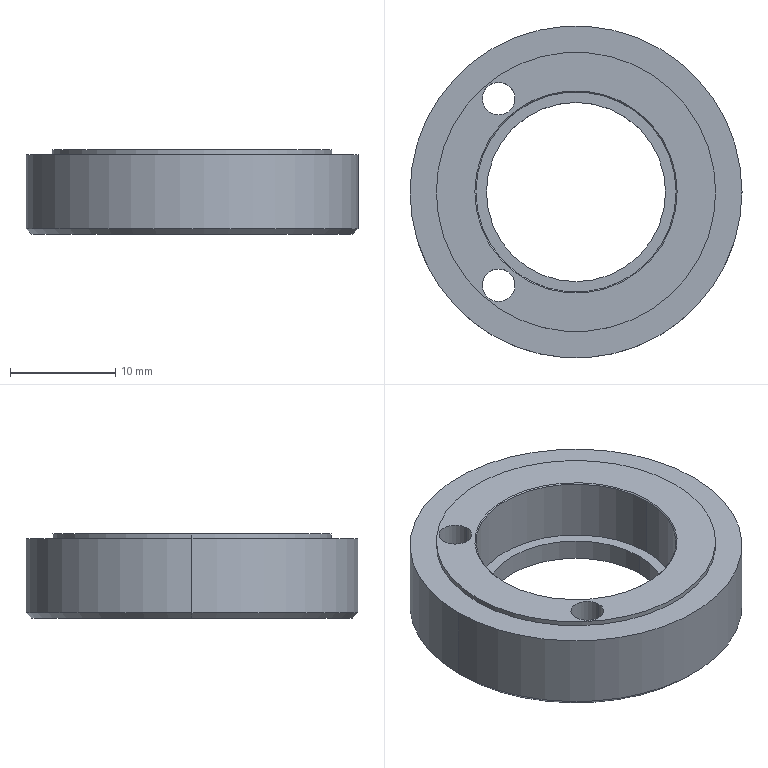Part | SolidWorks | features Chamfer 2, ICE 2, Extrusion 1, HoleWzd 1, MirrorPattern 1 | 1 solid | 20 faces | box 31.5 x 31.5 x 8 mm | volume 3844 mm3 | cylinder 12 | cone 4 | plane 4 | commonest cylinder face diameters 3.1 x4 17 x2 19 x2 26.5 x2 31.5 x2
STEP:
#1=CARTESIAN_POINT('',(-9.5,0.,3.9));
#2=VERTEX_POINT('',#1);
#3=CARTESIAN_POINT('',(9.5,0.,3.9));
#4=VERTEX_POINT('',#3);
#5=CARTESIAN_POINT('',(0.,0.,3.9));
#6=DIRECTION('',(0.,0.,1.));
#7=DIRECTION('',(1.,0.,0.));
#8=AXIS2_PLACEMENT_3D('',#5,#6,#7);
#9=CIRCLE('',#8,9.5);
#10=EDGE_CURVE('',#2,#4,#9,.T.);
#11=ORIENTED_EDGE('',*,*,#10,.F.);
#12=CARTESIAN_POINT('',(-9.6,0.,4.));
#13=VERTEX_POINT('',#12);
#14=CARTESIAN_POINT('',(-9.5,0.,3.9));
#15=DIRECTION('',(-0.7071,0.,0.7071));
#16=VECTOR('',#15,1000.);
#17=LINE('',#14,#16);
#18=EDGE_CURVE('',#2,#13,#17,.T.);
#19=ORIENTED_EDGE('',*,*,#18,.T.);
#20=CARTESIAN_POINT('',(9.6,0.,4.));
#21=VERTEX_POINT('',#20);
#22=CARTESIAN_POINT('',(0.,0.,4.));
#23=DIRECTION('',(0.,0.,-1.));
#24=DIRECTION('',(1.,0.,0.));
#25=AXIS2_PLACEMENT_3D('',#22,#23,#24);
#26=CIRCLE('',#25,9.6);
#27=EDGE_CURVE('',#21,#13,#26,.T.);
#28=ORIENTED_EDGE('',*,*,#27,.F.);
#29=CARTESIAN_POINT('',(9.5,0.,3.9));
#30=DIRECTION('',(0.7071,0.,0.7071));
#31=VECTOR('',#30,1000.);
#32=LINE('',#29,#31);
#33=EDGE_CURVE('',#4,#21,#32,.T.);
#34=ORIENTED_EDGE('',*,*,#33,.F.);
#35=EDGE_LOOP('',(#11,#19,#28,#34));
#36=FACE_OUTER_BOUND('',#35,.T.);
#37=CARTESIAN_POINT('',(0.,0.,3.9));
#38=DIRECTION('',(0.,0.,1.));
#39=DIRECTION('',(1.,0.,0.));
#40=AXIS2_PLACEMENT_3D('',#37,#38,#39);
#41=CONICAL_SURFACE('',#40,9.5,0.7854);
#42=ADVANCED_FACE('',(#36),#41,.F.);
#43=CARTESIAN_POINT('',(-15.25,0.,-4.));
#44=VERTEX_POINT('',#43);
#45=CARTESIAN_POINT('',(15.25,0.,-4.));
#46=VERTEX_POINT('',#45);
#47=CARTESIAN_POINT('',(0.,0.,-4.));
#48=DIRECTION('',(0.,0.,-1.));
#49=DIRECTION('',(1.,0.,0.));
#50=AXIS2_PLACEMENT_3D('',#47,#48,#49);
#51=CIRCLE('',#50,15.25);
#52=EDGE_CURVE('',#44,#46,#51,.T.);
#53=ORIENTED_EDGE('',*,*,#52,.F.);
#54=CARTESIAN_POINT('',(-15.75,0.,-3.5));
#55=VERTEX_POINT('',#54);
#56=CARTESIAN_POINT('',(-15.75,0.,-3.5));
#57=DIRECTION('',(-0.7071,0.,0.7071));
#58=VECTOR('',#57,1000.);
#59=LINE('',#56,#58);
#60=EDGE_CURVE('',#44,#55,#59,.T.);
#61=ORIENTED_EDGE('',*,*,#60,.T.);
#62=CARTESIAN_POINT('',(15.75,0.,-3.5));
#63=VERTEX_POINT('',#62);
#64=CARTESIAN_POINT('',(0.,0.,-3.5));
#65=DIRECTION('',(0.,0.,1.));
#66=DIRECTION('',(1.,0.,0.));
#67=AXIS2_PLACEMENT_3D('',#64,#65,#66);
#68=CIRCLE('',#67,15.75);
#69=EDGE_CURVE('',#63,#55,#68,.T.);
#70=ORIENTED_EDGE('',*,*,#69,.F.);
#71=CARTESIAN_POINT('',(15.75,0.,-3.5));
#72=DIRECTION('',(0.7071,0.,0.7071));
#73=VECTOR('',#72,1000.);
#74=LINE('',#71,#73);
#75=EDGE_CURVE('',#46,#63,#74,.T.);
#76=ORIENTED_EDGE('',*,*,#75,.F.);
#77=EDGE_LOOP('',(#53,#61,#70,#76));
#78=FACE_OUTER_BOUND('',#77,.T.);
#79=CARTESIAN_POINT('',(0.,0.,-3.5));
#80=DIRECTION('',(0.,0.,1.));
#81=DIRECTION('',(1.,0.,0.));
#82=AXIS2_PLACEMENT_3D('',#79,#80,#81);
#83=CONICAL_SURFACE('',#82,15.75,0.7854);
#84=ADVANCED_FACE('',(#78),#83,.T.);
#85=CARTESIAN_POINT('',(13.25,0.,3.55));
#86=VERTEX_POINT('',#85);
#87=CARTESIAN_POINT('',(-13.25,0.,3.55));
#88=VERTEX_POINT('',#87);
#89=CARTESIAN_POINT('',(0.,0.,3.55));
#90=DIRECTION('',(0.,0.,1.));
#91=DIRECTION('',(1.,0.,0.));
#92=AXIS2_PLACEMENT_3D('',#89,#90,#91);
#93=CIRCLE('',#92,13.25);
#94=EDGE_CURVE('',#86,#88,#93,.T.);
#95=ORIENTED_EDGE('',*,*,#94,.T.);
#96=CARTESIAN_POINT('',(-13.25,0.,4.));
#97=VERTEX_POINT('',#96);
#98=CARTESIAN_POINT('',(-13.25,0.,3.55));
#99=DIRECTION('',(0.,0.,1.));
#100=VECTOR('',#99,1000.);
#101=LINE('',#98,#100);
#102=EDGE_CURVE('',#88,#97,#101,.T.);
#103=ORIENTED_EDGE('',*,*,#102,.T.);
#104=CARTESIAN_POINT('',(13.25,0.,4.));
#105=VERTEX_POINT('',#104);
#106=CARTESIAN_POINT('',(0.,0.,4.));
#107=DIRECTION('',(0.,0.,1.));
#108=DIRECTION('',(1.,0.,0.));
#109=AXIS2_PLACEMENT_3D('',#106,#107,#108);
#110=CIRCLE('',#109,13.25);
#111=EDGE_CURVE('',#105,#97,#110,.T.);
#112=ORIENTED_EDGE('',*,*,#111,.F.);
#113=CARTESIAN_POINT('',(13.25,0.,3.55));
#114=DIRECTION('',(0.,0.,1.));
#115=VECTOR('',#114,1000.);
#116=LINE('',#113,#115);
#117=EDGE_CURVE('',#86,#105,#116,.T.);
#118=ORIENTED_EDGE('',*,*,#117,.F.);
#119=EDGE_LOOP('',(#95,#103,#112,#118));
#120=FACE_OUTER_BOUND('',#119,.T.);
#121=CARTESIAN_POINT('',(0.,0.,3.55));
#122=DIRECTION('',(0.,0.,1.));
#123=DIRECTION('',(1.,0.,0.));
#124=AXIS2_PLACEMENT_3D('',#121,#122,#123);
#125=CYLINDRICAL_SURFACE('',#124,13.25);
#126=ADVANCED_FACE('',(#120),#125,.T.);
#127=CARTESIAN_POINT('',(-5.792,-8.852,4.));
#128=VERTEX_POINT('',#127);
#129=CARTESIAN_POINT('',(-8.892,-8.852,4.));
#130=VERTEX_POINT('',#129);
#131=CARTESIAN_POINT('',(-7.342,-8.852,4.));
#132=DIRECTION('',(0.,0.,-1.));
#133=DIRECTION('',(-1.,0.,0.));
#134=AXIS2_PLACEMENT_3D('',#131,#132,#133);
#135=CIRCLE('',#134,1.55);
#136=EDGE_CURVE('',#128,#130,#135,.T.);
#137=ORIENTED_EDGE('',*,*,#136,.F.);
#138=CARTESIAN_POINT('',(-5.792,-8.852,-4.));
#139=VERTEX_POINT('',#138);
#140=CARTESIAN_POINT('',(-5.792,-8.852,-4.));
#141=DIRECTION('',(0.,0.,-1.));
#142=VECTOR('',#141,1000.);
#143=LINE('',#140,#142);
#144=EDGE_CURVE('',#128,#139,#143,.T.);
#145=ORIENTED_EDGE('',*,*,#144,.T.);
#146=CARTESIAN_POINT('',(-8.892,-8.852,-4.));
#147=VERTEX_POINT('',#146);
#148=CARTESIAN_POINT('',(-7.342,-8.852,-4.));
#149=DIRECTION('',(0.,0.,-1.));
#150=DIRECTION('',(-1.,0.,0.));
#151=AXIS2_PLACEMENT_3D('',#148,#149,#150);
#152=CIRCLE('',#151,1.55);
#153=EDGE_CURVE('',#139,#147,#152,.T.);
#154=ORIENTED_EDGE('',*,*,#153,.T.);
#155=CARTESIAN_POINT('',(-8.892,-8.852,-4.));
#156=DIRECTION('',(0.,0.,-1.));
#157=VECTOR('',#156,1000.);
#158=LINE('',#155,#157);
#159=EDGE_CURVE('',#130,#147,#158,.T.);
#160=ORIENTED_EDGE('',*,*,#159,.F.);
#161=EDGE_LOOP('',(#137,#145,#154,#160));
#162=FACE_OUTER_BOUND('',#161,.T.);
#163=CARTESIAN_POINT('',(-7.342,-8.852,-4.));
#164=DIRECTION('',(0.,0.,-1.));
#165=DIRECTION('',(-1.,0.,0.));
#166=AXIS2_PLACEMENT_3D('',#163,#164,#165);
#167=CYLINDRICAL_SURFACE('',#166,1.55);
#168=ADVANCED_FACE('',(#162),#167,.F.);
#169=CARTESIAN_POINT('',(-5.792,8.852,4.));
#170=VERTEX_POINT('',#169);
#171=CARTESIAN_POINT('',(-8.892,8.852,4.));
#172=VERTEX_POINT('',#171);
#173=CARTESIAN_POINT('',(-7.342,8.852,4.));
#174=DIRECTION('',(0.,0.,-1.));
#175=DIRECTION('',(-1.,0.,0.));
#176=AXIS2_PLACEMENT_3D('',#173,#174,#175);
#177=CIRCLE('',#176,1.55);
#178=EDGE_CURVE('',#170,#172,#177,.T.);
#179=ORIENTED_EDGE('',*,*,#178,.F.);
#180=CARTESIAN_POINT('',(-5.792,8.852,-4.));
#181=VERTEX_POINT('',#180);
#182=CARTESIAN_POINT('',(-5.792,8.852,-4.));
#183=DIRECTION('',(0.,0.,-1.));
#184=VECTOR('',#183,1000.);
#185=LINE('',#182,#184);
#186=EDGE_CURVE('',#170,#181,#185,.T.);
#187=ORIENTED_EDGE('',*,*,#186,.T.);
#188=CARTESIAN_POINT('',(-8.892,8.852,-4.));
#189=VERTEX_POINT('',#188);
#190=CARTESIAN_POINT('',(-7.342,8.852,-4.));
#191=DIRECTION('',(0.,0.,-1.));
#192=DIRECTION('',(-1.,0.,0.));
#193=AXIS2_PLACEMENT_3D('',#190,#191,#192);
#194=CIRCLE('',#193,1.55);
#195=EDGE_CURVE('',#181,#189,#194,.T.);
#196=ORIENTED_EDGE('',*,*,#195,.T.);
#197=CARTESIAN_POINT('',(-8.892,8.852,-4.));
#198=DIRECTION('',(0.,0.,-1.));
#199=VECTOR('',#198,1000.);
#200=LINE('',#197,#199);
#201=EDGE_CURVE('',#172,#189,#200,.T.);
#202=ORIENTED_EDGE('',*,*,#201,.F.);
#203=EDGE_LOOP('',(#179,#187,#196,#202));
#204=FACE_OUTER_BOUND('',#203,.T.);
#205=CARTESIAN_POINT('',(-7.342,8.852,-4.));
#206=DIRECTION('',(0.,0.,-1.));
#207=DIRECTION('',(-1.,0.,0.));
#208=AXIS2_PLACEMENT_3D('',#205,#206,#207);
#209=CYLINDRICAL_SURFACE('',#208,1.55);
#210=ADVANCED_FACE('',(#204),#209,.F.);
#211=CARTESIAN_POINT('',(8.5,0.,-2.));
#212=VERTEX_POINT('',#211);
#213=CARTESIAN_POINT('',(-8.5,0.,-2.));
#214=VERTEX_POINT('',#213);
#215=CARTESIAN_POINT('',(0.,0.,-2.));
#216=DIRECTION('',(0.,0.,-1.));
#217=DIRECTION('',(-1.,0.,0.));
#218=AXIS2_PLACEMENT_3D('',#215,#216,#217);
#219=CIRCLE('',#218,8.5);
#220=EDGE_CURVE('',#212,#214,#219,.T.);
#221=ORIENTED_EDGE('',*,*,#220,.F.);
#222=CARTESIAN_POINT('',(8.5,0.,-4.));
#223=VERTEX_POINT('',#222);
#224=CARTESIAN_POINT('',(8.5,0.,-2.));
#225=DIRECTION('',(0.,0.,-1.));
#226=VECTOR('',#225,1000.);
#227=LINE('',#224,#226);
#228=EDGE_CURVE('',#212,#223,#227,.T.);
#229=ORIENTED_EDGE('',*,*,#228,.T.);
#230=CARTESIAN_POINT('',(-8.5,0.,-4.));
#231=VERTEX_POINT('',#230);
#232=CARTESIAN_POINT('',(0.,0.,-4.));
#233=DIRECTION('',(0.,0.,-1.));
#234=DIRECTION('',(-1.,0.,0.));
#235=AXIS2_PLACEMENT_3D('',#232,#233,#234);
#236=CIRCLE('',#235,8.5);
#237=EDGE_CURVE('',#223,#231,#236,.T.);
#238=ORIENTED_EDGE('',*,*,#237,.T.);
#239=CARTESIAN_POINT('',(-8.5,0.,-2.));
#240=DIRECTION('',(0.,0.,-1.));
#241=VECTOR('',#240,1000.);
#242=LINE('',#239,#241);
#243=EDGE_CURVE('',#214,#231,#242,.T.);
#244=ORIENTED_EDGE('',*,*,#243,.F.);
#245=EDGE_LOOP('',(#221,#229,#238,#244));
#246=FACE_OUTER_BOUND('',#245,.T.);
#247=CARTESIAN_POINT('',(0.,0.,-2.));
#248=DIRECTION('',(0.,0.,-1.));
#249=DIRECTION('',(-1.,0.,0.));
#250=AXIS2_PLACEMENT_3D('',#247,#248,#249);
#251=CYLINDRICAL_SURFACE('',#250,8.5);
#252=ADVANCED_FACE('',(#246),#251,.F.);
#253=ORIENTED_EDGE('',*,*,#10,.T.);
#254=CARTESIAN_POINT('',(9.5,0.,-2.));
#255=VERTEX_POINT('',#254);
#256=CARTESIAN_POINT('',(9.5,0.,4.));
#257=DIRECTION('',(0.,0.,-1.));
#258=VECTOR('',#257,1000.);
#259=LINE('',#256,#258);
#260=EDGE_CURVE('',#4,#255,#259,.T.);
#261=ORIENTED_EDGE('',*,*,#260,.T.);
#262=CARTESIAN_POINT('',(-9.5,0.,-2.));
#263=VERTEX_POINT('',#262);
#264=CARTESIAN_POINT('',(0.,0.,-2.));
#265=DIRECTION('',(0.,0.,-1.));
#266=DIRECTION('',(-1.,0.,0.));
#267=AXIS2_PLACEMENT_3D('',#264,#265,#266);
#268=CIRCLE('',#267,9.5);
#269=EDGE_CURVE('',#255,#263,#268,.T.);
#270=ORIENTED_EDGE('',*,*,#269,.T.);
#271=CARTESIAN_POINT('',(-9.5,0.,4.));
#272=DIRECTION('',(0.,0.,-1.));
#273=VECTOR('',#272,1000.);
#274=LINE('',#271,#273);
#275=EDGE_CURVE('',#2,#263,#274,.T.);
#276=ORIENTED_EDGE('',*,*,#275,.F.);
#277=EDGE_LOOP('',(#253,#261,#270,#276));
#278=FACE_OUTER_BOUND('',#277,.T.);
#279=CARTESIAN_POINT('',(0.,0.,4.));
#280=DIRECTION('',(0.,0.,-1.));
#281=DIRECTION('',(-1.,0.,0.));
#282=AXIS2_PLACEMENT_3D('',#279,#280,#281);
#283=CYLINDRICAL_SURFACE('',#282,9.5);
#284=ADVANCED_FACE('',(#278),#283,.F.);
#285=CARTESIAN_POINT('',(15.75,0.,3.55));
#286=VERTEX_POINT('',#285);
#287=CARTESIAN_POINT('',(-15.75,0.,3.55));
#288=VERTEX_POINT('',#287);
#289=CARTESIAN_POINT('',(0.,0.,3.55));
#290=DIRECTION('',(0.,0.,1.));
#291=DIRECTION('',(1.,0.,0.));
#292=AXIS2_PLACEMENT_3D('',#289,#290,#291);
#293=CIRCLE('',#292,15.75);
#294=EDGE_CURVE('',#286,#288,#293,.T.);
#295=ORIENTED_EDGE('',*,*,#294,.F.);
#296=CARTESIAN_POINT('',(15.75,0.,4.));
#297=DIRECTION('',(0.,0.,-1.));
#298=VECTOR('',#297,1000.);
#299=LINE('',#296,#298);
#300=EDGE_CURVE('',#286,#63,#299,.T.);
#301=ORIENTED_EDGE('',*,*,#300,.T.);
#302=ORIENTED_EDGE('',*,*,#69,.T.);
#303=CARTESIAN_POINT('',(-15.75,0.,4.));
#304=DIRECTION('',(0.,0.,-1.));
#305=VECTOR('',#304,1000.);
#306=LINE('',#303,#305);
#307=EDGE_CURVE('',#288,#55,#306,.T.);
#308=ORIENTED_EDGE('',*,*,#307,.F.);
#309=EDGE_LOOP('',(#295,#301,#302,#308));
#310=FACE_OUTER_BOUND('',#309,.T.);
#311=CARTESIAN_POINT('',(0.,0.,4.));
#312=DIRECTION('',(0.,0.,-1.));
#313=DIRECTION('',(-1.,0.,0.));
#314=AXIS2_PLACEMENT_3D('',#311,#312,#313);
#315=CYLINDRICAL_SURFACE('',#314,15.75);
#316=ADVANCED_FACE('',(#310),#315,.T.);
#317=ORIENTED_EDGE('',*,*,#27,.T.);
#318=CARTESIAN_POINT('',(0.,0.,4.));
#319=DIRECTION('',(0.,0.,-1.));
#320=DIRECTION('',(1.,0.,0.));
#321=AXIS2_PLACEMENT_3D('',#318,#319,#320);
#322=CIRCLE('',#321,9.6);
#323=EDGE_CURVE('',#13,#21,#322,.T.);
#324=ORIENTED_EDGE('',*,*,#323,.T.);
#325=EDGE_LOOP('',(#317,#324));
#326=FACE_BOUND('',#325,.T.);
#327=CARTESIAN_POINT('',(-7.342,8.852,4.));
#328=DIRECTION('',(0.,0.,-1.));
#329=DIRECTION('',(-1.,0.,0.));
#330=AXIS2_PLACEMENT_3D('',#327,#328,#329);
#331=CIRCLE('',#330,1.55);
#332=EDGE_CURVE('',#172,#170,#331,.T.);
#333=ORIENTED_EDGE('',*,*,#332,.T.);
#334=ORIENTED_EDGE('',*,*,#178,.T.);
#335=EDGE_LOOP('',(#333,#334));
#336=FACE_BOUND('',#335,.T.);
#337=CARTESIAN_POINT('',(-7.342,-8.852,4.));
#338=DIRECTION('',(0.,0.,-1.));
#339=DIRECTION('',(-1.,0.,0.));
#340=AXIS2_PLACEMENT_3D('',#337,#338,#339);
#341=CIRCLE('',#340,1.55);
#342=EDGE_CURVE('',#130,#128,#341,.T.);
#343=ORIENTED_EDGE('',*,*,#342,.T.);
#344=ORIENTED_EDGE('',*,*,#136,.T.);
#345=EDGE_LOOP('',(#343,#344));
#346=FACE_BOUND('',#345,.T.);
#347=ORIENTED_EDGE('',*,*,#111,.T.);
#348=CARTESIAN_POINT('',(0.,0.,4.));
#349=DIRECTION('',(0.,0.,1.));
#350=DIRECTION('',(1.,0.,0.));
#351=AXIS2_PLACEMENT_3D('',#348,#349,#350);
#352=CIRCLE('',#351,13.25);
#353=EDGE_CURVE('',#97,#105,#352,.T.);
#354=ORIENTED_EDGE('',*,*,#353,.T.);
#355=EDGE_LOOP('',(#347,#354));
#356=FACE_OUTER_BOUND('',#355,.T.);
#357=CARTESIAN_POINT('',(0.,0.,4.));
#358=DIRECTION('',(0.,0.,1.));
#359=DIRECTION('',(1.,0.,0.));
#360=AXIS2_PLACEMENT_3D('',#357,#358,#359);
#361=PLANE('',#360);
#362=ADVANCED_FACE('',(#326,#336,#346,#356),#361,.T.);
#363=ORIENTED_EDGE('',*,*,#300,.F.);
#364=CARTESIAN_POINT('',(0.,0.,3.55));
#365=DIRECTION('',(0.,0.,1.));
#366=DIRECTION('',(1.,0.,0.));
#367=AXIS2_PLACEMENT_3D('',#364,#365,#366);
#368=CIRCLE('',#367,15.75);
#369=EDGE_CURVE('',#288,#286,#368,.T.);
#370=ORIENTED_EDGE('',*,*,#369,.F.);
#371=ORIENTED_EDGE('',*,*,#307,.T.);
#372=CARTESIAN_POINT('',(0.,0.,-3.5));
#373=DIRECTION('',(0.,0.,1.));
#374=DIRECTION('',(1.,0.,0.));
#375=AXIS2_PLACEMENT_3D('',#372,#373,#374);
#376=CIRCLE('',#375,15.75);
#377=EDGE_CURVE('',#55,#63,#376,.T.);
#378=ORIENTED_EDGE('',*,*,#377,.T.);
#379=EDGE_LOOP('',(#363,#370,#371,#378));
#380=FACE_OUTER_BOUND('',#379,.T.);
#381=CARTESIAN_POINT('',(0.,0.,4.));
#382=DIRECTION('',(0.,0.,-1.));
#383=DIRECTION('',(-1.,0.,0.));
#384=AXIS2_PLACEMENT_3D('',#381,#382,#383);
#385=CYLINDRICAL_SURFACE('',#384,15.75);
#386=ADVANCED_FACE('',(#380),#385,.T.);
#387=ORIENTED_EDGE('',*,*,#260,.F.);
#388=CARTESIAN_POINT('',(0.,0.,3.9));
#389=DIRECTION('',(0.,0.,1.));
#390=DIRECTION('',(1.,0.,0.));
#391=AXIS2_PLACEMENT_3D('',#388,#389,#390);
#392=CIRCLE('',#391,9.5);
#393=EDGE_CURVE('',#4,#2,#392,.T.);
#394=ORIENTED_EDGE('',*,*,#393,.T.);
#395=ORIENTED_EDGE('',*,*,#275,.T.);
#396=CARTESIAN_POINT('',(0.,0.,-2.));
#397=DIRECTION('',(0.,0.,-1.));
#398=DIRECTION('',(-1.,0.,0.));
#399=AXIS2_PLACEMENT_3D('',#396,#397,#398);
#400=CIRCLE('',#399,9.5);
#401=EDGE_CURVE('',#263,#255,#400,.T.);
#402=ORIENTED_EDGE('',*,*,#401,.T.);
#403=EDGE_LOOP('',(#387,#394,#395,#402));
#404=FACE_OUTER_BOUND('',#403,.T.);
#405=CARTESIAN_POINT('',(0.,0.,4.));
#406=DIRECTION('',(0.,0.,-1.));
#407=DIRECTION('',(-1.,0.,0.));
#408=AXIS2_PLACEMENT_3D('',#405,#406,#407);
#409=CYLINDRICAL_SURFACE('',#408,9.5);
#410=ADVANCED_FACE('',(#404),#409,.F.);
#411=CARTESIAN_POINT('',(0.,0.,-4.));
#412=DIRECTION('',(0.,0.,-1.));
#413=DIRECTION('',(1.,0.,0.));
#414=AXIS2_PLACEMENT_3D('',#411,#412,#413);
#415=CIRCLE('',#414,15.25);
#416=EDGE_CURVE('',#46,#44,#415,.T.);
#417=ORIENTED_EDGE('',*,*,#416,.T.);
#418=ORIENTED_EDGE('',*,*,#52,.T.);
#419=EDGE_LOOP('',(#417,#418));
#420=FACE_OUTER_BOUND('',#419,.T.);
#421=CARTESIAN_POINT('',(-7.342,-8.852,-4.));
#422=DIRECTION('',(0.,0.,-1.));
#423=DIRECTION('',(-1.,0.,0.));
#424=AXIS2_PLACEMENT_3D('',#421,#422,#423);
#425=CIRCLE('',#424,1.55);
#426=EDGE_CURVE('',#147,#139,#425,.T.);
#427=ORIENTED_EDGE('',*,*,#426,.F.);
#428=ORIENTED_EDGE('',*,*,#153,.F.);
#429=EDGE_LOOP('',(#427,#428));
#430=FACE_BOUND('',#429,.T.);
#431=CARTESIAN_POINT('',(-7.342,8.852,-4.));
#432=DIRECTION('',(0.,0.,-1.));
#433=DIRECTION('',(-1.,0.,0.));
#434=AXIS2_PLACEMENT_3D('',#431,#432,#433);
#435=CIRCLE('',#434,1.55);
#436=EDGE_CURVE('',#189,#181,#435,.T.);
#437=ORIENTED_EDGE('',*,*,#436,.F.);
#438=ORIENTED_EDGE('',*,*,#195,.F.);
#439=EDGE_LOOP('',(#437,#438));
#440=FACE_BOUND('',#439,.T.);
#441=CARTESIAN_POINT('',(0.,0.,-4.));
#442=DIRECTION('',(0.,0.,-1.));
#443=DIRECTION('',(-1.,0.,0.));
#444=AXIS2_PLACEMENT_3D('',#441,#442,#443);
#445=CIRCLE('',#444,8.5);
#446=EDGE_CURVE('',#231,#223,#445,.T.);
#447=ORIENTED_EDGE('',*,*,#446,.F.);
#448=ORIENTED_EDGE('',*,*,#237,.F.);
#449=EDGE_LOOP('',(#447,#448));
#450=FACE_BOUND('',#449,.T.);
#451=CARTESIAN_POINT('',(0.,0.,-4.));
#452=DIRECTION('',(0.,0.,1.));
#453=DIRECTION('',(1.,0.,0.));
#454=AXIS2_PLACEMENT_3D('',#451,#452,#453);
#455=PLANE('',#454);
#456=ADVANCED_FACE('',(#420,#430,#440,#450),#455,.F.);
#457=CARTESIAN_POINT('',(0.,0.,-2.));
#458=DIRECTION('',(0.,0.,-1.));
#459=DIRECTION('',(-1.,0.,0.));
#460=AXIS2_PLACEMENT_3D('',#457,#458,#459);
#461=CIRCLE('',#460,8.5);
#462=EDGE_CURVE('',#214,#212,#461,.T.);
#463=ORIENTED_EDGE('',*,*,#462,.T.);
#464=ORIENTED_EDGE('',*,*,#220,.T.);
#465=EDGE_LOOP('',(#463,#464));
#466=FACE_BOUND('',#465,.T.);
#467=ORIENTED_EDGE('',*,*,#401,.F.);
#468=ORIENTED_EDGE('',*,*,#269,.F.);
#469=EDGE_LOOP('',(#467,#468));
#470=FACE_OUTER_BOUND('',#469,.T.);
#471=CARTESIAN_POINT('',(0.,0.,-2.));
#472=DIRECTION('',(0.,0.,-1.));
#473=DIRECTION('',(-1.,0.,0.));
#474=AXIS2_PLACEMENT_3D('',#471,#472,#473);
#475=PLANE('',#474);
#476=ADVANCED_FACE('',(#466,#470),#475,.F.);
#477=ORIENTED_EDGE('',*,*,#228,.F.);
#478=ORIENTED_EDGE('',*,*,#462,.F.);
#479=ORIENTED_EDGE('',*,*,#243,.T.);
#480=ORIENTED_EDGE('',*,*,#446,.T.);
#481=EDGE_LOOP('',(#477,#478,#479,#480));
#482=FACE_OUTER_BOUND('',#481,.T.);
#483=CARTESIAN_POINT('',(0.,0.,-2.));
#484=DIRECTION('',(0.,0.,-1.));
#485=DIRECTION('',(-1.,0.,0.));
#486=AXIS2_PLACEMENT_3D('',#483,#484,#485);
#487=CYLINDRICAL_SURFACE('',#486,8.5);
#488=ADVANCED_FACE('',(#482),#487,.F.);
#489=ORIENTED_EDGE('',*,*,#186,.F.);
#490=ORIENTED_EDGE('',*,*,#332,.F.);
#491=ORIENTED_EDGE('',*,*,#201,.T.);
#492=ORIENTED_EDGE('',*,*,#436,.T.);
#493=EDGE_LOOP('',(#489,#490,#491,#492));
#494=FACE_OUTER_BOUND('',#493,.T.);
#495=CARTESIAN_POINT('',(-7.342,8.852,-4.));
#496=DIRECTION('',(0.,0.,-1.));
#497=DIRECTION('',(-1.,0.,0.));
#498=AXIS2_PLACEMENT_3D('',#495,#496,#497);
#499=CYLINDRICAL_SURFACE('',#498,1.55);
#500=ADVANCED_FACE('',(#494),#499,.F.);
#501=ORIENTED_EDGE('',*,*,#144,.F.);
#502=ORIENTED_EDGE('',*,*,#342,.F.);
#503=ORIENTED_EDGE('',*,*,#159,.T.);
#504=ORIENTED_EDGE('',*,*,#426,.T.);
#505=EDGE_LOOP('',(#501,#502,#503,#504));
#506=FACE_OUTER_BOUND('',#505,.T.);
#507=CARTESIAN_POINT('',(-7.342,-8.852,-4.));
#508=DIRECTION('',(0.,0.,-1.));
#509=DIRECTION('',(-1.,0.,0.));
#510=AXIS2_PLACEMENT_3D('',#507,#508,#509);
#511=CYLINDRICAL_SURFACE('',#510,1.55);
#512=ADVANCED_FACE('',(#506),#511,.F.);
#513=ORIENTED_EDGE('',*,*,#94,.F.);
#514=CARTESIAN_POINT('',(0.,0.,3.55));
#515=DIRECTION('',(0.,0.,1.));
#516=DIRECTION('',(1.,0.,0.));
#517=AXIS2_PLACEMENT_3D('',#514,#515,#516);
#518=CIRCLE('',#517,13.25);
#519=EDGE_CURVE('',#88,#86,#518,.T.);
#520=ORIENTED_EDGE('',*,*,#519,.F.);
#521=EDGE_LOOP('',(#513,#520));
#522=FACE_BOUND('',#521,.T.);
#523=ORIENTED_EDGE('',*,*,#369,.T.);
#524=ORIENTED_EDGE('',*,*,#294,.T.);
#525=EDGE_LOOP('',(#523,#524));
#526=FACE_OUTER_BOUND('',#525,.T.);
#527=CARTESIAN_POINT('',(0.,0.,3.55));
#528=DIRECTION('',(0.,0.,1.));
#529=DIRECTION('',(1.,0.,0.));
#530=AXIS2_PLACEMENT_3D('',#527,#528,#529);
#531=PLANE('',#530);
#532=ADVANCED_FACE('',(#522,#526),#531,.T.);
#533=ORIENTED_EDGE('',*,*,#102,.F.);
#534=ORIENTED_EDGE('',*,*,#519,.T.);
#535=ORIENTED_EDGE('',*,*,#117,.T.);
#536=ORIENTED_EDGE('',*,*,#353,.F.);
#537=EDGE_LOOP('',(#533,#534,#535,#536));
#538=FACE_OUTER_BOUND('',#537,.T.);
#539=CARTESIAN_POINT('',(0.,0.,3.55));
#540=DIRECTION('',(0.,0.,1.));
#541=DIRECTION('',(1.,0.,0.));
#542=AXIS2_PLACEMENT_3D('',#539,#540,#541);
#543=CYLINDRICAL_SURFACE('',#542,13.25);
#544=ADVANCED_FACE('',(#538),#543,.T.);
#545=ORIENTED_EDGE('',*,*,#60,.F.);
#546=ORIENTED_EDGE('',*,*,#416,.F.);
#547=ORIENTED_EDGE('',*,*,#75,.T.);
#548=ORIENTED_EDGE('',*,*,#377,.F.);
#549=EDGE_LOOP('',(#545,#546,#547,#548));
#550=FACE_OUTER_BOUND('',#549,.T.);
#551=CARTESIAN_POINT('',(0.,0.,-3.5));
#552=DIRECTION('',(0.,0.,1.));
#553=DIRECTION('',(1.,0.,0.));
#554=AXIS2_PLACEMENT_3D('',#551,#552,#553);
#555=CONICAL_SURFACE('',#554,15.75,0.7854);
#556=ADVANCED_FACE('',(#550),#555,.T.);
#557=ORIENTED_EDGE('',*,*,#18,.F.);
#558=ORIENTED_EDGE('',*,*,#393,.F.);
#559=ORIENTED_EDGE('',*,*,#33,.T.);
#560=ORIENTED_EDGE('',*,*,#323,.F.);
#561=EDGE_LOOP('',(#557,#558,#559,#560));
#562=FACE_OUTER_BOUND('',#561,.T.);
#563=CARTESIAN_POINT('',(0.,0.,3.9));
#564=DIRECTION('',(0.,0.,1.));
#565=DIRECTION('',(1.,0.,0.));
#566=AXIS2_PLACEMENT_3D('',#563,#564,#565);
#567=CONICAL_SURFACE('',#566,9.5,0.7854);
#568=ADVANCED_FACE('',(#562),#567,.F.);
#569=CLOSED_SHELL('',(#42,#84,#126,#168,#210,#252,#284,#316,#362,#386,#410,#456,#476,#488,#500,#512,#532,#544,#556,#568));
#570=MANIFOLD_SOLID_BREP('',#569);
#571=CARTESIAN_POINT('',(0.,0.,0.));
#572=DIRECTION('',(0.,0.,1.));
#573=DIRECTION('',(1.,0.,0.));
#574=AXIS2_PLACEMENT_3D('',#571,#572,#573);
#575=(LENGTH_UNIT()NAMED_UNIT(*)SI_UNIT(.MILLI.,.METRE.));
#576=UNCERTAINTY_MEASURE_WITH_UNIT(LENGTH_MEASURE(0.00001),#575,'','');
#577=(NAMED_UNIT(*)PLANE_ANGLE_UNIT()SI_UNIT($,.RADIAN.));
#578=(NAMED_UNIT(*)SI_UNIT($,.STERADIAN.)SOLID_ANGLE_UNIT());
#579=(GEOMETRIC_REPRESENTATION_CONTEXT(3)GLOBAL_UNCERTAINTY_ASSIGNED_CONTEXT((#576))GLOBAL_UNIT_ASSIGNED_CONTEXT((#575,#577,#578))REPRESENTATION_CONTEXT('',''));
#580=ADVANCED_BREP_SHAPE_REPRESENTATION('',(#570,#574),#579);